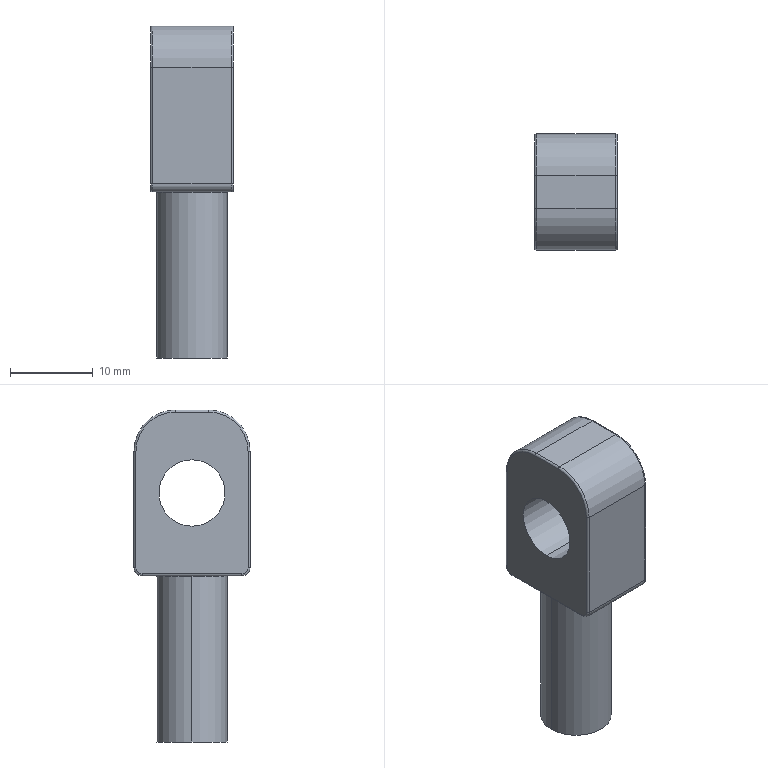Part | SolidWorks | features Cut 1, Extrusion 1, Fillet 1, HoleWzd 1, ICE 1 | 2 solids | 38 faces | box 10 x 14 x 40.005 mm | volume 3250 mm3 | cylinder 18 | plane 8 | torus 8 | cone 4 | commonest cylinder face diameters 0.5 x8 2 x2 2.9 x2 8 x2 8.5 x2 10 x2
STEP:
#1=CARTESIAN_POINT('',(1.45,0.,0.325));
#2=VERTEX_POINT('',#1);
#3=CARTESIAN_POINT('',(-1.45,0.,0.325));
#4=VERTEX_POINT('',#3);
#5=CARTESIAN_POINT('',(0.,0.,0.325));
#6=DIRECTION('',(0.,0.,-1.));
#7=DIRECTION('',(-1.,0.,0.));
#8=AXIS2_PLACEMENT_3D('',#5,#6,#7);
#9=CIRCLE('',#8,1.45);
#10=EDGE_CURVE('',#2,#4,#9,.T.);
#11=ORIENTED_EDGE('',*,*,#10,.F.);
#12=CARTESIAN_POINT('',(1.775,0.,0.));
#13=VERTEX_POINT('',#12);
#14=CARTESIAN_POINT('',(1.775,0.,0.));
#15=DIRECTION('',(0.7071,0.,-0.7071));
#16=VECTOR('',#15,1000.);
#17=LINE('',#14,#16);
#18=EDGE_CURVE('',#2,#13,#17,.T.);
#19=ORIENTED_EDGE('',*,*,#18,.T.);
#20=CARTESIAN_POINT('',(-1.775,0.,0.));
#21=VERTEX_POINT('',#20);
#22=CARTESIAN_POINT('',(0.,0.,0.));
#23=DIRECTION('',(0.,0.,-1.));
#24=DIRECTION('',(-1.,0.,0.));
#25=AXIS2_PLACEMENT_3D('',#22,#23,#24);
#26=CIRCLE('',#25,1.775);
#27=EDGE_CURVE('',#13,#21,#26,.T.);
#28=ORIENTED_EDGE('',*,*,#27,.T.);
#29=CARTESIAN_POINT('',(-1.775,0.,0.));
#30=DIRECTION('',(-0.7071,0.,-0.7071));
#31=VECTOR('',#30,1000.);
#32=LINE('',#29,#31);
#33=EDGE_CURVE('',#4,#21,#32,.T.);
#34=ORIENTED_EDGE('',*,*,#33,.F.);
#35=EDGE_LOOP('',(#11,#19,#28,#34));
#36=FACE_OUTER_BOUND('',#35,.T.);
#37=CARTESIAN_POINT('',(0.,0.,0.));
#38=DIRECTION('',(0.,0.,-1.));
#39=DIRECTION('',(-1.,0.,0.));
#40=AXIS2_PLACEMENT_3D('',#37,#38,#39);
#41=CONICAL_SURFACE('',#40,1.775,0.7854);
#42=ADVANCED_FACE('',(#36),#41,.F.);
#43=CARTESIAN_POINT('',(1.45,0.,10.));
#44=VERTEX_POINT('',#43);
#45=CARTESIAN_POINT('',(-1.45,0.,10.));
#46=VERTEX_POINT('',#45);
#47=CARTESIAN_POINT('',(0.,0.,10.));
#48=DIRECTION('',(0.,0.,-1.));
#49=DIRECTION('',(-1.,0.,0.));
#50=AXIS2_PLACEMENT_3D('',#47,#48,#49);
#51=CIRCLE('',#50,1.45);
#52=EDGE_CURVE('',#44,#46,#51,.T.);
#53=ORIENTED_EDGE('',*,*,#52,.F.);
#54=CARTESIAN_POINT('',(1.45,0.,0.));
#55=DIRECTION('',(0.,0.,-1.));
#56=VECTOR('',#55,1000.);
#57=LINE('',#54,#56);
#58=EDGE_CURVE('',#44,#2,#57,.T.);
#59=ORIENTED_EDGE('',*,*,#58,.T.);
#60=ORIENTED_EDGE('',*,*,#10,.T.);
#61=CARTESIAN_POINT('',(-1.45,0.,0.));
#62=DIRECTION('',(0.,0.,-1.));
#63=VECTOR('',#62,1000.);
#64=LINE('',#61,#63);
#65=EDGE_CURVE('',#46,#4,#64,.T.);
#66=ORIENTED_EDGE('',*,*,#65,.F.);
#67=EDGE_LOOP('',(#53,#59,#60,#66));
#68=FACE_OUTER_BOUND('',#67,.T.);
#69=CARTESIAN_POINT('',(0.,0.,0.));
#70=DIRECTION('',(0.,0.,-1.));
#71=DIRECTION('',(-1.,0.,0.));
#72=AXIS2_PLACEMENT_3D('',#69,#70,#71);
#73=CYLINDRICAL_SURFACE('',#72,1.45);
#74=ADVANCED_FACE('',(#68),#73,.F.);
#75=CARTESIAN_POINT('',(0.,0.,10.871));
#76=VERTEX_POINT('',#75);
#77=CARTESIAN_POINT('',(-1.45,0.,10.));
#78=DIRECTION('',(-0.8572,0.,-0.515));
#79=VECTOR('',#78,1000.);
#80=LINE('',#77,#79);
#81=EDGE_CURVE('',#76,#46,#80,.T.);
#82=ORIENTED_EDGE('',*,*,#81,.F.);
#83=CARTESIAN_POINT('',(1.45,0.,10.));
#84=DIRECTION('',(0.8572,0.,-0.515));
#85=VECTOR('',#84,1000.);
#86=LINE('',#83,#85);
#87=EDGE_CURVE('',#76,#44,#86,.T.);
#88=ORIENTED_EDGE('',*,*,#87,.T.);
#89=ORIENTED_EDGE('',*,*,#52,.T.);
#90=EDGE_LOOP('',(#82,#88,#89));
#91=FACE_OUTER_BOUND('',#90,.T.);
#92=CARTESIAN_POINT('',(0.,0.,10.));
#93=DIRECTION('',(0.,0.,-1.));
#94=DIRECTION('',(-1.,0.,0.));
#95=AXIS2_PLACEMENT_3D('',#92,#93,#94);
#96=CONICAL_SURFACE('',#95,1.45,1.03);
#97=ADVANCED_FACE('',(#91),#96,.F.);
#98=CARTESIAN_POINT('',(4.25,0.,20.));
#99=VERTEX_POINT('',#98);
#100=CARTESIAN_POINT('',(-4.25,0.,20.));
#101=VERTEX_POINT('',#100);
#102=CARTESIAN_POINT('',(0.,0.,20.));
#103=DIRECTION('',(0.,0.,1.));
#104=DIRECTION('',(1.,0.,0.));
#105=AXIS2_PLACEMENT_3D('',#102,#103,#104);
#106=CIRCLE('',#105,4.25);
#107=EDGE_CURVE('',#99,#101,#106,.T.);
#108=ORIENTED_EDGE('',*,*,#107,.F.);
#109=CARTESIAN_POINT('',(4.25,0.,0.));
#110=VERTEX_POINT('',#109);
#111=CARTESIAN_POINT('',(4.25,0.,20.));
#112=DIRECTION('',(0.,0.,-1.));
#113=VECTOR('',#112,1000.);
#114=LINE('',#111,#113);
#115=EDGE_CURVE('',#99,#110,#114,.T.);
#116=ORIENTED_EDGE('',*,*,#115,.T.);
#117=CARTESIAN_POINT('',(-4.25,0.,0.));
#118=VERTEX_POINT('',#117);
#119=CARTESIAN_POINT('',(0.,0.,0.));
#120=DIRECTION('',(0.,0.,1.));
#121=DIRECTION('',(1.,0.,0.));
#122=AXIS2_PLACEMENT_3D('',#119,#120,#121);
#123=CIRCLE('',#122,4.25);
#124=EDGE_CURVE('',#110,#118,#123,.T.);
#125=ORIENTED_EDGE('',*,*,#124,.T.);
#126=CARTESIAN_POINT('',(-4.25,0.,20.));
#127=DIRECTION('',(0.,0.,-1.));
#128=VECTOR('',#127,1000.);
#129=LINE('',#126,#128);
#130=EDGE_CURVE('',#101,#118,#129,.T.);
#131=ORIENTED_EDGE('',*,*,#130,.F.);
#132=EDGE_LOOP('',(#108,#116,#125,#131));
#133=FACE_OUTER_BOUND('',#132,.T.);
#134=CARTESIAN_POINT('',(0.,0.,20.));
#135=DIRECTION('',(0.,0.,-1.));
#136=DIRECTION('',(-1.,0.,0.));
#137=AXIS2_PLACEMENT_3D('',#134,#135,#136);
#138=CYLINDRICAL_SURFACE('',#137,4.25);
#139=ADVANCED_FACE('',(#133),#138,.T.);
#140=ORIENTED_EDGE('',*,*,#115,.F.);
#141=CARTESIAN_POINT('',(0.,0.,20.));
#142=DIRECTION('',(0.,0.,1.));
#143=DIRECTION('',(1.,0.,0.));
#144=AXIS2_PLACEMENT_3D('',#141,#142,#143);
#145=CIRCLE('',#144,4.25);
#146=EDGE_CURVE('',#101,#99,#145,.T.);
#147=ORIENTED_EDGE('',*,*,#146,.F.);
#148=ORIENTED_EDGE('',*,*,#130,.T.);
#149=CARTESIAN_POINT('',(0.,0.,0.));
#150=DIRECTION('',(0.,0.,1.));
#151=DIRECTION('',(1.,0.,0.));
#152=AXIS2_PLACEMENT_3D('',#149,#150,#151);
#153=CIRCLE('',#152,4.25);
#154=EDGE_CURVE('',#118,#110,#153,.T.);
#155=ORIENTED_EDGE('',*,*,#154,.T.);
#156=EDGE_LOOP('',(#140,#147,#148,#155));
#157=FACE_OUTER_BOUND('',#156,.T.);
#158=CARTESIAN_POINT('',(0.,0.,20.));
#159=DIRECTION('',(0.,0.,-1.));
#160=DIRECTION('',(-1.,0.,0.));
#161=AXIS2_PLACEMENT_3D('',#158,#159,#160);
#162=CYLINDRICAL_SURFACE('',#161,4.25);
#163=ADVANCED_FACE('',(#157),#162,.T.);
#164=ORIENTED_EDGE('',*,*,#146,.T.);
#165=ORIENTED_EDGE('',*,*,#107,.T.);
#166=EDGE_LOOP('',(#164,#165));
#167=FACE_OUTER_BOUND('',#166,.T.);
#168=CARTESIAN_POINT('',(0.,0.,20.));
#169=DIRECTION('',(0.,0.,1.));
#170=DIRECTION('',(1.,0.,0.));
#171=AXIS2_PLACEMENT_3D('',#168,#169,#170);
#172=PLANE('',#171);
#173=ADVANCED_FACE('',(#167),#172,.T.);
#174=CARTESIAN_POINT('',(0.,0.,0.));
#175=DIRECTION('',(0.,0.,-1.));
#176=DIRECTION('',(-1.,0.,0.));
#177=AXIS2_PLACEMENT_3D('',#174,#175,#176);
#178=CIRCLE('',#177,1.775);
#179=EDGE_CURVE('',#21,#13,#178,.T.);
#180=ORIENTED_EDGE('',*,*,#179,.F.);
#181=ORIENTED_EDGE('',*,*,#27,.F.);
#182=EDGE_LOOP('',(#180,#181));
#183=FACE_BOUND('',#182,.T.);
#184=ORIENTED_EDGE('',*,*,#154,.F.);
#185=ORIENTED_EDGE('',*,*,#124,.F.);
#186=EDGE_LOOP('',(#184,#185));
#187=FACE_OUTER_BOUND('',#186,.T.);
#188=CARTESIAN_POINT('',(0.,0.,0.));
#189=DIRECTION('',(0.,0.,1.));
#190=DIRECTION('',(1.,0.,0.));
#191=AXIS2_PLACEMENT_3D('',#188,#189,#190);
#192=PLANE('',#191);
#193=ADVANCED_FACE('',(#183,#187),#192,.F.);
#194=ORIENTED_EDGE('',*,*,#87,.F.);
#195=ORIENTED_EDGE('',*,*,#81,.T.);
#196=CARTESIAN_POINT('',(0.,0.,10.));
#197=DIRECTION('',(0.,0.,-1.));
#198=DIRECTION('',(-1.,0.,0.));
#199=AXIS2_PLACEMENT_3D('',#196,#197,#198);
#200=CIRCLE('',#199,1.45);
#201=EDGE_CURVE('',#46,#44,#200,.T.);
#202=ORIENTED_EDGE('',*,*,#201,.T.);
#203=EDGE_LOOP('',(#194,#195,#202));
#204=FACE_OUTER_BOUND('',#203,.T.);
#205=CARTESIAN_POINT('',(0.,0.,10.));
#206=DIRECTION('',(0.,0.,-1.));
#207=DIRECTION('',(-1.,0.,0.));
#208=AXIS2_PLACEMENT_3D('',#205,#206,#207);
#209=CONICAL_SURFACE('',#208,1.45,1.03);
#210=ADVANCED_FACE('',(#204),#209,.F.);
#211=ORIENTED_EDGE('',*,*,#58,.F.);
#212=ORIENTED_EDGE('',*,*,#201,.F.);
#213=ORIENTED_EDGE('',*,*,#65,.T.);
#214=CARTESIAN_POINT('',(0.,0.,0.325));
#215=DIRECTION('',(0.,0.,-1.));
#216=DIRECTION('',(-1.,0.,0.));
#217=AXIS2_PLACEMENT_3D('',#214,#215,#216);
#218=CIRCLE('',#217,1.45);
#219=EDGE_CURVE('',#4,#2,#218,.T.);
#220=ORIENTED_EDGE('',*,*,#219,.T.);
#221=EDGE_LOOP('',(#211,#212,#213,#220));
#222=FACE_OUTER_BOUND('',#221,.T.);
#223=CARTESIAN_POINT('',(0.,0.,0.));
#224=DIRECTION('',(0.,0.,-1.));
#225=DIRECTION('',(-1.,0.,0.));
#226=AXIS2_PLACEMENT_3D('',#223,#224,#225);
#227=CYLINDRICAL_SURFACE('',#226,1.45);
#228=ADVANCED_FACE('',(#222),#227,.F.);
#229=ORIENTED_EDGE('',*,*,#18,.F.);
#230=ORIENTED_EDGE('',*,*,#219,.F.);
#231=ORIENTED_EDGE('',*,*,#33,.T.);
#232=ORIENTED_EDGE('',*,*,#179,.T.);
#233=EDGE_LOOP('',(#229,#230,#231,#232));
#234=FACE_OUTER_BOUND('',#233,.T.);
#235=CARTESIAN_POINT('',(0.,0.,0.));
#236=DIRECTION('',(0.,0.,-1.));
#237=DIRECTION('',(-1.,0.,0.));
#238=AXIS2_PLACEMENT_3D('',#235,#236,#237);
#239=CONICAL_SURFACE('',#238,1.775,0.7854);
#240=ADVANCED_FACE('',(#234),#239,.F.);
#241=CLOSED_SHELL('',(#42,#74,#97,#139,#163,#173,#193,#210,#228,#240));
#242=MANIFOLD_SOLID_BREP('',#241);
#243=CARTESIAN_POINT('',(-5.,0.,34.005));
#244=VERTEX_POINT('',#243);
#245=CARTESIAN_POINT('',(-5.,0.,26.005));
#246=VERTEX_POINT('',#245);
#247=CARTESIAN_POINT('',(-5.,0.,30.005));
#248=DIRECTION('',(1.,0.,0.));
#249=DIRECTION('',(0.,0.,1.));
#250=AXIS2_PLACEMENT_3D('',#247,#248,#249);
#251=CIRCLE('',#250,4.);
#252=EDGE_CURVE('',#244,#246,#251,.T.);
#253=ORIENTED_EDGE('',*,*,#252,.F.);
#254=CARTESIAN_POINT('',(5.,0.,34.005));
#255=VERTEX_POINT('',#254);
#256=CARTESIAN_POINT('',(-5.001,0.,34.005));
#257=DIRECTION('',(1.,0.,0.));
#258=VECTOR('',#257,1000.);
#259=LINE('',#256,#258);
#260=EDGE_CURVE('',#244,#255,#259,.T.);
#261=ORIENTED_EDGE('',*,*,#260,.T.);
#262=CARTESIAN_POINT('',(5.,0.,26.005));
#263=VERTEX_POINT('',#262);
#264=CARTESIAN_POINT('',(5.,0.,30.005));
#265=DIRECTION('',(1.,0.,0.));
#266=DIRECTION('',(0.,0.,-1.));
#267=AXIS2_PLACEMENT_3D('',#264,#265,#266);
#268=CIRCLE('',#267,4.);
#269=EDGE_CURVE('',#255,#263,#268,.T.);
#270=ORIENTED_EDGE('',*,*,#269,.T.);
#271=CARTESIAN_POINT('',(-5.001,0.,26.005));
#272=DIRECTION('',(1.,0.,0.));
#273=VECTOR('',#272,1000.);
#274=LINE('',#271,#273);
#275=EDGE_CURVE('',#246,#263,#274,.T.);
#276=ORIENTED_EDGE('',*,*,#275,.F.);
#277=EDGE_LOOP('',(#253,#261,#270,#276));
#278=FACE_OUTER_BOUND('',#277,.T.);
#279=CARTESIAN_POINT('',(-5.001,0.,30.005));
#280=DIRECTION('',(1.,0.,0.));
#281=DIRECTION('',(0.,0.,-1.));
#282=AXIS2_PLACEMENT_3D('',#279,#280,#281);
#283=CYLINDRICAL_SURFACE('',#282,4.);
#284=ADVANCED_FACE('',(#278),#283,.F.);
#285=CARTESIAN_POINT('',(4.75,-2.,40.005));
#286=VERTEX_POINT('',#285);
#287=CARTESIAN_POINT('',(-4.75,-2.,40.005));
#288=VERTEX_POINT('',#287);
#289=CARTESIAN_POINT('',(5.,-2.,40.005));
#290=DIRECTION('',(-1.,0.,0.));
#291=VECTOR('',#290,1000.);
#292=LINE('',#289,#291);
#293=EDGE_CURVE('',#286,#288,#292,.T.);
#294=ORIENTED_EDGE('',*,*,#293,.T.);
#295=CARTESIAN_POINT('',(-4.75,-7.,35.005));
#296=VERTEX_POINT('',#295);
#297=CARTESIAN_POINT('',(-4.75,-2.,35.005));
#298=DIRECTION('',(1.,0.,0.));
#299=DIRECTION('',(0.,0.,1.));
#300=AXIS2_PLACEMENT_3D('',#297,#298,#299);
#301=CIRCLE('',#300,5.);
#302=EDGE_CURVE('',#288,#296,#301,.T.);
#303=ORIENTED_EDGE('',*,*,#302,.T.);
#304=CARTESIAN_POINT('',(4.75,-7.,35.005));
#305=VERTEX_POINT('',#304);
#306=CARTESIAN_POINT('',(5.,-7.,35.005));
#307=DIRECTION('',(-1.,0.,0.));
#308=VECTOR('',#307,1000.);
#309=LINE('',#306,#308);
#310=EDGE_CURVE('',#305,#296,#309,.T.);
#311=ORIENTED_EDGE('',*,*,#310,.F.);
#312=CARTESIAN_POINT('',(4.75,-2.,35.005));
#313=DIRECTION('',(-1.,0.,0.));
#314=DIRECTION('',(0.,0.,1.));
#315=AXIS2_PLACEMENT_3D('',#312,#313,#314);
#316=CIRCLE('',#315,5.);
#317=EDGE_CURVE('',#305,#286,#316,.T.);
#318=ORIENTED_EDGE('',*,*,#317,.T.);
#319=EDGE_LOOP('',(#294,#303,#311,#318));
#320=FACE_OUTER_BOUND('',#319,.T.);
#321=CARTESIAN_POINT('',(5.,-2.,35.005));
#322=DIRECTION('',(-1.,0.,0.));
#323=DIRECTION('',(0.,0.,1.));
#324=AXIS2_PLACEMENT_3D('',#321,#322,#323);
#325=CYLINDRICAL_SURFACE('',#324,5.);
#326=ADVANCED_FACE('',(#320),#325,.T.);
#327=ORIENTED_EDGE('',*,*,#310,.T.);
#328=CARTESIAN_POINT('',(-4.75,-7.,21.005));
#329=VERTEX_POINT('',#328);
#330=CARTESIAN_POINT('',(-4.75,-7.,21.005));
#331=DIRECTION('',(0.,0.,-1.));
#332=VECTOR('',#331,1000.);
#333=LINE('',#330,#332);
#334=EDGE_CURVE('',#296,#329,#333,.T.);
#335=ORIENTED_EDGE('',*,*,#334,.T.);
#336=CARTESIAN_POINT('',(4.75,-7.,21.005));
#337=VERTEX_POINT('',#336);
#338=CARTESIAN_POINT('',(5.,-7.,21.005));
#339=DIRECTION('',(-1.,0.,0.));
#340=VECTOR('',#339,1000.);
#341=LINE('',#338,#340);
#342=EDGE_CURVE('',#337,#329,#341,.T.);
#343=ORIENTED_EDGE('',*,*,#342,.F.);
#344=CARTESIAN_POINT('',(4.75,-7.,21.005));
#345=DIRECTION('',(0.,0.,1.));
#346=VECTOR('',#345,1000.);
#347=LINE('',#344,#346);
#348=EDGE_CURVE('',#337,#305,#347,.T.);
#349=ORIENTED_EDGE('',*,*,#348,.T.);
#350=EDGE_LOOP('',(#327,#335,#343,#349));
#351=FACE_OUTER_BOUND('',#350,.T.);
#352=CARTESIAN_POINT('',(5.,-7.,21.005));
#353=DIRECTION('',(0.,1.,0.));
#354=DIRECTION('',(0.,0.,1.));
#355=AXIS2_PLACEMENT_3D('',#352,#353,#354);
#356=PLANE('',#355);
#357=ADVANCED_FACE('',(#351),#356,.F.);
#358=ORIENTED_EDGE('',*,*,#342,.T.);
#359=CARTESIAN_POINT('',(-4.75,-6.,20.005));
#360=VERTEX_POINT('',#359);
#361=CARTESIAN_POINT('',(-4.75,-6.,21.005));
#362=DIRECTION('',(1.,0.,0.));
#363=DIRECTION('',(0.,0.,1.));
#364=AXIS2_PLACEMENT_3D('',#361,#362,#363);
#365=CIRCLE('',#364,1.);
#366=EDGE_CURVE('',#329,#360,#365,.T.);
#367=ORIENTED_EDGE('',*,*,#366,.T.);
#368=CARTESIAN_POINT('',(4.75,-6.,20.005));
#369=VERTEX_POINT('',#368);
#370=CARTESIAN_POINT('',(5.,-6.,20.005));
#371=DIRECTION('',(-1.,0.,0.));
#372=VECTOR('',#371,1000.);
#373=LINE('',#370,#372);
#374=EDGE_CURVE('',#369,#360,#373,.T.);
#375=ORIENTED_EDGE('',*,*,#374,.F.);
#376=CARTESIAN_POINT('',(4.75,-6.,21.005));
#377=DIRECTION('',(-1.,0.,0.));
#378=DIRECTION('',(0.,0.,1.));
#379=AXIS2_PLACEMENT_3D('',#376,#377,#378);
#380=CIRCLE('',#379,1.);
#381=EDGE_CURVE('',#369,#337,#380,.T.);
#382=ORIENTED_EDGE('',*,*,#381,.T.);
#383=EDGE_LOOP('',(#358,#367,#375,#382));
#384=FACE_OUTER_BOUND('',#383,.T.);
#385=CARTESIAN_POINT('',(5.,-6.,21.005));
#386=DIRECTION('',(-1.,0.,0.));
#387=DIRECTION('',(0.,0.,1.));
#388=AXIS2_PLACEMENT_3D('',#385,#386,#387);
#389=CYLINDRICAL_SURFACE('',#388,1.);
#390=ADVANCED_FACE('',(#384),#389,.T.);
#391=ORIENTED_EDGE('',*,*,#374,.T.);
#392=CARTESIAN_POINT('',(-4.75,6.,20.005));
#393=VERTEX_POINT('',#392);
#394=CARTESIAN_POINT('',(-4.75,6.,20.005));
#395=DIRECTION('',(0.,1.,0.));
#396=VECTOR('',#395,1000.);
#397=LINE('',#394,#396);
#398=EDGE_CURVE('',#360,#393,#397,.T.);
#399=ORIENTED_EDGE('',*,*,#398,.T.);
#400=CARTESIAN_POINT('',(4.75,6.,20.005));
#401=VERTEX_POINT('',#400);
#402=CARTESIAN_POINT('',(5.,6.,20.005));
#403=DIRECTION('',(-1.,0.,0.));
#404=VECTOR('',#403,1000.);
#405=LINE('',#402,#404);
#406=EDGE_CURVE('',#401,#393,#405,.T.);
#407=ORIENTED_EDGE('',*,*,#406,.F.);
#408=CARTESIAN_POINT('',(4.75,-6.,20.005));
#409=DIRECTION('',(0.,-1.,0.));
#410=VECTOR('',#409,1000.);
#411=LINE('',#408,#410);
#412=EDGE_CURVE('',#401,#369,#411,.T.);
#413=ORIENTED_EDGE('',*,*,#412,.T.);
#414=EDGE_LOOP('',(#391,#399,#407,#413));
#415=FACE_OUTER_BOUND('',#414,.T.);
#416=CARTESIAN_POINT('',(5.,-6.,20.005));
#417=DIRECTION('',(0.,0.,1.));
#418=DIRECTION('',(1.,0.,0.));
#419=AXIS2_PLACEMENT_3D('',#416,#417,#418);
#420=PLANE('',#419);
#421=ADVANCED_FACE('',(#415),#420,.F.);
#422=ORIENTED_EDGE('',*,*,#406,.T.);
#423=CARTESIAN_POINT('',(-4.75,7.,21.005));
#424=VERTEX_POINT('',#423);
#425=CARTESIAN_POINT('',(-4.75,6.,21.005));
#426=DIRECTION('',(1.,0.,0.));
#427=DIRECTION('',(0.,0.,1.));
#428=AXIS2_PLACEMENT_3D('',#425,#426,#427);
#429=CIRCLE('',#428,1.);
#430=EDGE_CURVE('',#393,#424,#429,.T.);
#431=ORIENTED_EDGE('',*,*,#430,.T.);
#432=CARTESIAN_POINT('',(4.75,7.,21.005));
#433=VERTEX_POINT('',#432);
#434=CARTESIAN_POINT('',(5.,7.,21.005));
#435=DIRECTION('',(-1.,0.,0.));
#436=VECTOR('',#435,1000.);
#437=LINE('',#434,#436);
#438=EDGE_CURVE('',#433,#424,#437,.T.);
#439=ORIENTED_EDGE('',*,*,#438,.F.);
#440=CARTESIAN_POINT('',(4.75,6.,21.005));
#441=DIRECTION('',(-1.,0.,0.));
#442=DIRECTION('',(0.,0.,1.));
#443=AXIS2_PLACEMENT_3D('',#440,#441,#442);
#444=CIRCLE('',#443,1.);
#445=EDGE_CURVE('',#433,#401,#444,.T.);
#446=ORIENTED_EDGE('',*,*,#445,.T.);
#447=EDGE_LOOP('',(#422,#431,#439,#446));
#448=FACE_OUTER_BOUND('',#447,.T.);
#449=CARTESIAN_POINT('',(5.,6.,21.005));
#450=DIRECTION('',(-1.,0.,0.));
#451=DIRECTION('',(0.,0.,1.));
#452=AXIS2_PLACEMENT_3D('',#449,#450,#451);
#453=CYLINDRICAL_SURFACE('',#452,1.);
#454=ADVANCED_FACE('',(#448),#453,.T.);
#455=ORIENTED_EDGE('',*,*,#438,.T.);
#456=CARTESIAN_POINT('',(-4.75,7.,35.005));
#457=VERTEX_POINT('',#456);
#458=CARTESIAN_POINT('',(-4.75,7.,35.005));
#459=DIRECTION('',(0.,0.,1.));
#460=VECTOR('',#459,1000.);
#461=LINE('',#458,#460);
#462=EDGE_CURVE('',#424,#457,#461,.T.);
#463=ORIENTED_EDGE('',*,*,#462,.T.);
#464=CARTESIAN_POINT('',(4.75,7.,35.005));
#465=VERTEX_POINT('',#464);
#466=CARTESIAN_POINT('',(5.,7.,35.005));
#467=DIRECTION('',(-1.,0.,0.));
#468=VECTOR('',#467,1000.);
#469=LINE('',#466,#468);
#470=EDGE_CURVE('',#465,#457,#469,.T.);
#471=ORIENTED_EDGE('',*,*,#470,.F.);
#472=CARTESIAN_POINT('',(4.75,7.,21.005));
#473=DIRECTION('',(0.,0.,-1.));
#474=VECTOR('',#473,1000.);
#475=LINE('',#472,#474);
#476=EDGE_CURVE('',#465,#433,#475,.T.);
#477=ORIENTED_EDGE('',*,*,#476,.T.);
#478=EDGE_LOOP('',(#455,#463,#471,#477));
#479=FACE_OUTER_BOUND('',#478,.T.);
#480=CARTESIAN_POINT('',(5.,7.,21.005));
#481=DIRECTION('',(0.,-1.,0.));
#482=DIRECTION('',(0.,0.,-1.));
#483=AXIS2_PLACEMENT_3D('',#480,#481,#482);
#484=PLANE('',#483);
#485=ADVANCED_FACE('',(#479),#484,.F.);
#486=ORIENTED_EDGE('',*,*,#470,.T.);
#487=CARTESIAN_POINT('',(-4.75,2.,40.005));
#488=VERTEX_POINT('',#487);
#489=CARTESIAN_POINT('',(-4.75,2.,35.005));
#490=DIRECTION('',(1.,0.,0.));
#491=DIRECTION('',(0.,0.,1.));
#492=AXIS2_PLACEMENT_3D('',#489,#490,#491);
#493=CIRCLE('',#492,5.);
#494=EDGE_CURVE('',#457,#488,#493,.T.);
#495=ORIENTED_EDGE('',*,*,#494,.T.);
#496=CARTESIAN_POINT('',(4.75,2.,40.005));
#497=VERTEX_POINT('',#496);
#498=CARTESIAN_POINT('',(5.,2.,40.005));
#499=DIRECTION('',(-1.,0.,0.));
#500=VECTOR('',#499,1000.);
#501=LINE('',#498,#500);
#502=EDGE_CURVE('',#497,#488,#501,.T.);
#503=ORIENTED_EDGE('',*,*,#502,.F.);
#504=CARTESIAN_POINT('',(4.75,2.,35.005));
#505=DIRECTION('',(-1.,0.,0.));
#506=DIRECTION('',(0.,0.,1.));
#507=AXIS2_PLACEMENT_3D('',#504,#505,#506);
#508=CIRCLE('',#507,5.);
#509=EDGE_CURVE('',#497,#465,#508,.T.);
#510=ORIENTED_EDGE('',*,*,#509,.T.);
#511=EDGE_LOOP('',(#486,#495,#503,#510));
#512=FACE_OUTER_BOUND('',#511,.T.);
#513=CARTESIAN_POINT('',(5.,2.,35.005));
#514=DIRECTION('',(-1.,0.,0.));
#515=DIRECTION('',(0.,0.,1.));
#516=AXIS2_PLACEMENT_3D('',#513,#514,#515);
#517=CYLINDRICAL_SURFACE('',#516,5.);
#518=ADVANCED_FACE('',(#512),#517,.T.);
#519=ORIENTED_EDGE('',*,*,#502,.T.);
#520=CARTESIAN_POINT('',(-4.75,-2.,40.005));
#521=DIRECTION('',(0.,-1.,0.));
#522=VECTOR('',#521,1000.);
#523=LINE('',#520,#522);
#524=EDGE_CURVE('',#488,#288,#523,.T.);
#525=ORIENTED_EDGE('',*,*,#524,.T.);
#526=ORIENTED_EDGE('',*,*,#293,.F.);
#527=CARTESIAN_POINT('',(4.75,-2.,40.005));
#528=DIRECTION('',(0.,1.,0.));
#529=VECTOR('',#528,1000.);
#530=LINE('',#527,#529);
#531=EDGE_CURVE('',#286,#497,#530,.T.);
#532=ORIENTED_EDGE('',*,*,#531,.T.);
#533=EDGE_LOOP('',(#519,#525,#526,#532));
#534=FACE_OUTER_BOUND('',#533,.T.);
#535=CARTESIAN_POINT('',(5.,-2.,40.005));
#536=DIRECTION('',(0.,0.,-1.));
#537=DIRECTION('',(-1.,0.,0.));
#538=AXIS2_PLACEMENT_3D('',#535,#536,#537);
#539=PLANE('',#538);
#540=ADVANCED_FACE('',(#534),#539,.F.);
#541=CARTESIAN_POINT('',(5.,0.,30.005));
#542=DIRECTION('',(1.,0.,0.));
#543=DIRECTION('',(0.,0.,-1.));
#544=AXIS2_PLACEMENT_3D('',#541,#542,#543);
#545=CIRCLE('',#544,4.);
#546=EDGE_CURVE('',#263,#255,#545,.T.);
#547=ORIENTED_EDGE('',*,*,#546,.F.);
#548=ORIENTED_EDGE('',*,*,#269,.F.);
#549=EDGE_LOOP('',(#547,#548));
#550=FACE_BOUND('',#549,.T.);
#551=CARTESIAN_POINT('',(5.,6.75,35.005));
#552=VERTEX_POINT('',#551);
#553=CARTESIAN_POINT('',(5.,2.,39.755));
#554=VERTEX_POINT('',#553);
#555=CARTESIAN_POINT('',(5.,2.,35.005));
#556=DIRECTION('',(1.,0.,0.));
#557=DIRECTION('',(0.,0.,1.));
#558=AXIS2_PLACEMENT_3D('',#555,#556,#557);
#559=CIRCLE('',#558,4.75);
#560=EDGE_CURVE('',#552,#554,#559,.T.);
#561=ORIENTED_EDGE('',*,*,#560,.T.);
#562=CARTESIAN_POINT('',(5.,-2.,39.755));
#563=VERTEX_POINT('',#562);
#564=CARTESIAN_POINT('',(5.,-2.,39.755));
#565=DIRECTION('',(0.,-1.,0.));
#566=VECTOR('',#565,1000.);
#567=LINE('',#564,#566);
#568=EDGE_CURVE('',#554,#563,#567,.T.);
#569=ORIENTED_EDGE('',*,*,#568,.T.);
#570=CARTESIAN_POINT('',(5.,-6.75,35.005));
#571=VERTEX_POINT('',#570);
#572=CARTESIAN_POINT('',(5.,-2.,35.005));
#573=DIRECTION('',(1.,0.,0.));
#574=DIRECTION('',(0.,0.,1.));
#575=AXIS2_PLACEMENT_3D('',#572,#573,#574);
#576=CIRCLE('',#575,4.75);
#577=EDGE_CURVE('',#563,#571,#576,.T.);
#578=ORIENTED_EDGE('',*,*,#577,.T.);
#579=CARTESIAN_POINT('',(5.,-6.75,21.005));
#580=VERTEX_POINT('',#579);
#581=CARTESIAN_POINT('',(5.,-6.75,35.005));
#582=DIRECTION('',(0.,0.,-1.));
#583=VECTOR('',#582,1000.);
#584=LINE('',#581,#583);
#585=EDGE_CURVE('',#571,#580,#584,.T.);
#586=ORIENTED_EDGE('',*,*,#585,.T.);
#587=CARTESIAN_POINT('',(5.,-6.,20.255));
#588=VERTEX_POINT('',#587);
#589=CARTESIAN_POINT('',(5.,-6.,21.005));
#590=DIRECTION('',(1.,0.,0.));
#591=DIRECTION('',(0.,0.,1.));
#592=AXIS2_PLACEMENT_3D('',#589,#590,#591);
#593=CIRCLE('',#592,0.75);
#594=EDGE_CURVE('',#580,#588,#593,.T.);
#595=ORIENTED_EDGE('',*,*,#594,.T.);
#596=CARTESIAN_POINT('',(5.,6.,20.255));
#597=VERTEX_POINT('',#596);
#598=CARTESIAN_POINT('',(5.,-2.,20.255));
#599=DIRECTION('',(0.,1.,0.));
#600=VECTOR('',#599,1000.);
#601=LINE('',#598,#600);
#602=EDGE_CURVE('',#588,#597,#601,.T.);
#603=ORIENTED_EDGE('',*,*,#602,.T.);
#604=CARTESIAN_POINT('',(5.,6.75,21.005));
#605=VERTEX_POINT('',#604);
#606=CARTESIAN_POINT('',(5.,6.,21.005));
#607=DIRECTION('',(1.,0.,0.));
#608=DIRECTION('',(0.,0.,1.));
#609=AXIS2_PLACEMENT_3D('',#606,#607,#608);
#610=CIRCLE('',#609,0.75);
#611=EDGE_CURVE('',#597,#605,#610,.T.);
#612=ORIENTED_EDGE('',*,*,#611,.T.);
#613=CARTESIAN_POINT('',(5.,6.75,35.005));
#614=DIRECTION('',(0.,0.,1.));
#615=VECTOR('',#614,1000.);
#616=LINE('',#613,#615);
#617=EDGE_CURVE('',#605,#552,#616,.T.);
#618=ORIENTED_EDGE('',*,*,#617,.T.);
#619=EDGE_LOOP('',(#561,#569,#578,#586,#595,#603,#612,#618));
#620=FACE_OUTER_BOUND('',#619,.T.);
#621=CARTESIAN_POINT('',(5.,-2.,35.005));
#622=DIRECTION('',(-1.,0.,0.));
#623=DIRECTION('',(0.,0.,1.));
#624=AXIS2_PLACEMENT_3D('',#621,#622,#623);
#625=PLANE('',#624);
#626=ADVANCED_FACE('',(#550,#620),#625,.F.);
#627=CARTESIAN_POINT('',(-5.,0.,30.005));
#628=DIRECTION('',(1.,0.,0.));
#629=DIRECTION('',(0.,0.,1.));
#630=AXIS2_PLACEMENT_3D('',#627,#628,#629);
#631=CIRCLE('',#630,4.);
#632=EDGE_CURVE('',#246,#244,#631,.T.);
#633=ORIENTED_EDGE('',*,*,#632,.T.);
#634=ORIENTED_EDGE('',*,*,#252,.T.);
#635=EDGE_LOOP('',(#633,#634));
#636=FACE_BOUND('',#635,.T.);
#637=CARTESIAN_POINT('',(-5.,-6.,20.255));
#638=VERTEX_POINT('',#637);
#639=CARTESIAN_POINT('',(-5.,-6.75,21.005));
#640=VERTEX_POINT('',#639);
#641=CARTESIAN_POINT('',(-5.,-6.,21.005));
#642=DIRECTION('',(-1.,0.,0.));
#643=DIRECTION('',(0.,0.,1.));
#644=AXIS2_PLACEMENT_3D('',#641,#642,#643);
#645=CIRCLE('',#644,0.75);
#646=EDGE_CURVE('',#638,#640,#645,.T.);
#647=ORIENTED_EDGE('',*,*,#646,.T.);
#648=CARTESIAN_POINT('',(-5.,-6.75,35.005));
#649=VERTEX_POINT('',#648);
#650=CARTESIAN_POINT('',(-5.,-6.75,35.005));
#651=DIRECTION('',(0.,0.,1.));
#652=VECTOR('',#651,1000.);
#653=LINE('',#650,#652);
#654=EDGE_CURVE('',#640,#649,#653,.T.);
#655=ORIENTED_EDGE('',*,*,#654,.T.);
#656=CARTESIAN_POINT('',(-5.,-2.,39.755));
#657=VERTEX_POINT('',#656);
#658=CARTESIAN_POINT('',(-5.,-2.,35.005));
#659=DIRECTION('',(-1.,0.,0.));
#660=DIRECTION('',(0.,0.,1.));
#661=AXIS2_PLACEMENT_3D('',#658,#659,#660);
#662=CIRCLE('',#661,4.75);
#663=EDGE_CURVE('',#649,#657,#662,.T.);
#664=ORIENTED_EDGE('',*,*,#663,.T.);
#665=CARTESIAN_POINT('',(-5.,2.,39.755));
#666=VERTEX_POINT('',#665);
#667=CARTESIAN_POINT('',(-5.,2.,39.755));
#668=DIRECTION('',(0.,1.,0.));
#669=VECTOR('',#668,1000.);
#670=LINE('',#667,#669);
#671=EDGE_CURVE('',#657,#666,#670,.T.);
#672=ORIENTED_EDGE('',*,*,#671,.T.);
#673=CARTESIAN_POINT('',(-5.,6.75,35.005));
#674=VERTEX_POINT('',#673);
#675=CARTESIAN_POINT('',(-5.,2.,35.005));
#676=DIRECTION('',(-1.,0.,0.));
#677=DIRECTION('',(0.,0.,1.));
#678=AXIS2_PLACEMENT_3D('',#675,#676,#677);
#679=CIRCLE('',#678,4.75);
#680=EDGE_CURVE('',#666,#674,#679,.T.);
#681=ORIENTED_EDGE('',*,*,#680,.T.);
#682=CARTESIAN_POINT('',(-5.,6.75,21.005));
#683=VERTEX_POINT('',#682);
#684=CARTESIAN_POINT('',(-5.,6.75,21.005));
#685=DIRECTION('',(0.,0.,-1.));
#686=VECTOR('',#685,1000.);
#687=LINE('',#684,#686);
#688=EDGE_CURVE('',#674,#683,#687,.T.);
#689=ORIENTED_EDGE('',*,*,#688,.T.);
#690=CARTESIAN_POINT('',(-5.,6.,20.255));
#691=VERTEX_POINT('',#690);
#692=CARTESIAN_POINT('',(-5.,6.,21.005));
#693=DIRECTION('',(-1.,0.,0.));
#694=DIRECTION('',(0.,0.,1.));
#695=AXIS2_PLACEMENT_3D('',#692,#693,#694);
#696=CIRCLE('',#695,0.75);
#697=EDGE_CURVE('',#683,#691,#696,.T.);
#698=ORIENTED_EDGE('',*,*,#697,.T.);
#699=CARTESIAN_POINT('',(-5.,-6.,20.255));
#700=DIRECTION('',(0.,-1.,0.));
#701=VECTOR('',#700,1000.);
#702=LINE('',#699,#701);
#703=EDGE_CURVE('',#691,#638,#702,.T.);
#704=ORIENTED_EDGE('',*,*,#703,.T.);
#705=EDGE_LOOP('',(#647,#655,#664,#672,#681,#689,#698,#704));
#706=FACE_OUTER_BOUND('',#705,.T.);
#707=CARTESIAN_POINT('',(-5.,-2.,35.005));
#708=DIRECTION('',(-1.,0.,0.));
#709=DIRECTION('',(0.,0.,1.));
#710=AXIS2_PLACEMENT_3D('',#707,#708,#709);
#711=PLANE('',#710);
#712=ADVANCED_FACE('',(#636,#706),#711,.T.);
#713=CARTESIAN_POINT('',(-4.75,6.75,21.005));
#714=DIRECTION('',(0.,0.,-1.));
#715=DIRECTION('',(0.,1.,0.));
#716=AXIS2_PLACEMENT_3D('',#713,#714,#715);
#717=CIRCLE('',#716,0.25);
#718=EDGE_CURVE('',#683,#424,#717,.T.);
#719=ORIENTED_EDGE('',*,*,#718,.F.);
#720=ORIENTED_EDGE('',*,*,#688,.F.);
#721=CARTESIAN_POINT('',(-4.75,6.75,35.005));
#722=DIRECTION('',(0.,0.,1.));
#723=DIRECTION('',(1.,0.,0.));
#724=AXIS2_PLACEMENT_3D('',#721,#722,#723);
#725=CIRCLE('',#724,0.25);
#726=EDGE_CURVE('',#457,#674,#725,.T.);
#727=ORIENTED_EDGE('',*,*,#726,.F.);
#728=ORIENTED_EDGE('',*,*,#462,.F.);
#729=EDGE_LOOP('',(#719,#720,#727,#728));
#730=FACE_OUTER_BOUND('',#729,.T.);
#731=CARTESIAN_POINT('',(-4.75,6.75,21.005));
#732=DIRECTION('',(0.,0.,-1.));
#733=DIRECTION('',(0.,1.,0.));
#734=AXIS2_PLACEMENT_3D('',#731,#732,#733);
#735=CYLINDRICAL_SURFACE('',#734,0.25);
#736=ADVANCED_FACE('',(#730),#735,.T.);
#737=ORIENTED_EDGE('',*,*,#726,.T.);
#738=ORIENTED_EDGE('',*,*,#680,.F.);
#739=CARTESIAN_POINT('',(-4.75,2.,39.755));
#740=DIRECTION('',(0.,-1.,0.));
#741=DIRECTION('',(0.,0.,-1.));
#742=AXIS2_PLACEMENT_3D('',#739,#740,#741);
#743=CIRCLE('',#742,0.25);
#744=EDGE_CURVE('',#488,#666,#743,.T.);
#745=ORIENTED_EDGE('',*,*,#744,.F.);
#746=ORIENTED_EDGE('',*,*,#494,.F.);
#747=EDGE_LOOP('',(#737,#738,#745,#746));
#748=FACE_OUTER_BOUND('',#747,.T.);
#749=CARTESIAN_POINT('',(-4.75,2.,35.005));
#750=DIRECTION('',(-1.,0.,0.));
#751=DIRECTION('',(0.,0.,1.));
#752=AXIS2_PLACEMENT_3D('',#749,#750,#751);
#753=TOROIDAL_SURFACE('',#752,4.75,0.25);
#754=ADVANCED_FACE('',(#748),#753,.T.);
#755=ORIENTED_EDGE('',*,*,#718,.T.);
#756=ORIENTED_EDGE('',*,*,#430,.F.);
#757=CARTESIAN_POINT('',(-4.75,6.,20.255));
#758=DIRECTION('',(0.,-1.,0.));
#759=DIRECTION('',(0.,0.,-1.));
#760=AXIS2_PLACEMENT_3D('',#757,#758,#759);
#761=CIRCLE('',#760,0.25);
#762=EDGE_CURVE('',#691,#393,#761,.T.);
#763=ORIENTED_EDGE('',*,*,#762,.F.);
#764=ORIENTED_EDGE('',*,*,#697,.F.);
#765=EDGE_LOOP('',(#755,#756,#763,#764));
#766=FACE_OUTER_BOUND('',#765,.T.);
#767=CARTESIAN_POINT('',(-4.75,6.,21.005));
#768=DIRECTION('',(-1.,0.,0.));
#769=DIRECTION('',(0.,0.,1.));
#770=AXIS2_PLACEMENT_3D('',#767,#768,#769);
#771=TOROIDAL_SURFACE('',#770,0.75,0.25);
#772=ADVANCED_FACE('',(#766),#771,.T.);
#773=ORIENTED_EDGE('',*,*,#744,.T.);
#774=ORIENTED_EDGE('',*,*,#671,.F.);
#775=CARTESIAN_POINT('',(-4.75,-2.,39.755));
#776=DIRECTION('',(0.,-1.,0.));
#777=DIRECTION('',(0.,0.,-1.));
#778=AXIS2_PLACEMENT_3D('',#775,#776,#777);
#779=CIRCLE('',#778,0.25);
#780=EDGE_CURVE('',#288,#657,#779,.T.);
#781=ORIENTED_EDGE('',*,*,#780,.F.);
#782=ORIENTED_EDGE('',*,*,#524,.F.);
#783=EDGE_LOOP('',(#773,#774,#781,#782));
#784=FACE_OUTER_BOUND('',#783,.T.);
#785=CARTESIAN_POINT('',(-4.75,-2.,39.755));
#786=DIRECTION('',(0.,1.,0.));
#787=DIRECTION('',(0.,0.,1.));
#788=AXIS2_PLACEMENT_3D('',#785,#786,#787);
#789=CYLINDRICAL_SURFACE('',#788,0.25);
#790=ADVANCED_FACE('',(#784),#789,.T.);
#791=ORIENTED_EDGE('',*,*,#762,.T.);
#792=ORIENTED_EDGE('',*,*,#398,.F.);
#793=CARTESIAN_POINT('',(-4.75,-6.,20.255));
#794=DIRECTION('',(0.,-1.,0.));
#795=DIRECTION('',(0.,0.,-1.));
#796=AXIS2_PLACEMENT_3D('',#793,#794,#795);
#797=CIRCLE('',#796,0.25);
#798=EDGE_CURVE('',#638,#360,#797,.T.);
#799=ORIENTED_EDGE('',*,*,#798,.F.);
#800=ORIENTED_EDGE('',*,*,#703,.F.);
#801=EDGE_LOOP('',(#791,#792,#799,#800));
#802=FACE_OUTER_BOUND('',#801,.T.);
#803=CARTESIAN_POINT('',(-4.75,-6.,20.255));
#804=DIRECTION('',(0.,-1.,0.));
#805=DIRECTION('',(0.,0.,-1.));
#806=AXIS2_PLACEMENT_3D('',#803,#804,#805);
#807=CYLINDRICAL_SURFACE('',#806,0.25);
#808=ADVANCED_FACE('',(#802),#807,.T.);
#809=ORIENTED_EDGE('',*,*,#780,.T.);
#810=ORIENTED_EDGE('',*,*,#663,.F.);
#811=CARTESIAN_POINT('',(-4.75,-6.75,35.005));
#812=DIRECTION('',(0.,0.,-1.));
#813=DIRECTION('',(-1.,0.,0.));
#814=AXIS2_PLACEMENT_3D('',#811,#812,#813);
#815=CIRCLE('',#814,0.25);
#816=EDGE_CURVE('',#296,#649,#815,.T.);
#817=ORIENTED_EDGE('',*,*,#816,.F.);
#818=ORIENTED_EDGE('',*,*,#302,.F.);
#819=EDGE_LOOP('',(#809,#810,#817,#818));
#820=FACE_OUTER_BOUND('',#819,.T.);
#821=CARTESIAN_POINT('',(-4.75,-2.,35.005));
#822=DIRECTION('',(-1.,0.,0.));
#823=DIRECTION('',(0.,0.,1.));
#824=AXIS2_PLACEMENT_3D('',#821,#822,#823);
#825=TOROIDAL_SURFACE('',#824,4.75,0.25);
#826=ADVANCED_FACE('',(#820),#825,.T.);
#827=ORIENTED_EDGE('',*,*,#798,.T.);
#828=ORIENTED_EDGE('',*,*,#366,.F.);
#829=CARTESIAN_POINT('',(-4.75,-6.75,21.005));
#830=DIRECTION('',(0.,0.,1.));
#831=DIRECTION('',(1.,0.,0.));
#832=AXIS2_PLACEMENT_3D('',#829,#830,#831);
#833=CIRCLE('',#832,0.25);
#834=EDGE_CURVE('',#640,#329,#833,.T.);
#835=ORIENTED_EDGE('',*,*,#834,.F.);
#836=ORIENTED_EDGE('',*,*,#646,.F.);
#837=EDGE_LOOP('',(#827,#828,#835,#836));
#838=FACE_OUTER_BOUND('',#837,.T.);
#839=CARTESIAN_POINT('',(-4.75,-6.,21.005));
#840=DIRECTION('',(-1.,0.,0.));
#841=DIRECTION('',(0.,0.,1.));
#842=AXIS2_PLACEMENT_3D('',#839,#840,#841);
#843=TOROIDAL_SURFACE('',#842,0.75,0.25);
#844=ADVANCED_FACE('',(#838),#843,.T.);
#845=ORIENTED_EDGE('',*,*,#816,.T.);
#846=ORIENTED_EDGE('',*,*,#654,.F.);
#847=ORIENTED_EDGE('',*,*,#834,.T.);
#848=ORIENTED_EDGE('',*,*,#334,.F.);
#849=EDGE_LOOP('',(#845,#846,#847,#848));
#850=FACE_OUTER_BOUND('',#849,.T.);
#851=CARTESIAN_POINT('',(-4.75,-6.75,21.005));
#852=DIRECTION('',(0.,0.,1.));
#853=DIRECTION('',(0.,-1.,0.));
#854=AXIS2_PLACEMENT_3D('',#851,#852,#853);
#855=CYLINDRICAL_SURFACE('',#854,0.25);
#856=ADVANCED_FACE('',(#850),#855,.T.);
#857=CARTESIAN_POINT('',(4.75,-6.,20.255));
#858=DIRECTION('',(0.,-1.,0.));
#859=DIRECTION('',(0.,0.,-1.));
#860=AXIS2_PLACEMENT_3D('',#857,#858,#859);
#861=CIRCLE('',#860,0.25);
#862=EDGE_CURVE('',#369,#588,#861,.T.);
#863=ORIENTED_EDGE('',*,*,#862,.F.);
#864=ORIENTED_EDGE('',*,*,#412,.F.);
#865=CARTESIAN_POINT('',(4.75,6.,20.255));
#866=DIRECTION('',(0.,1.,0.));
#867=DIRECTION('',(0.,0.,1.));
#868=AXIS2_PLACEMENT_3D('',#865,#866,#867);
#869=CIRCLE('',#868,0.25);
#870=EDGE_CURVE('',#597,#401,#869,.T.);
#871=ORIENTED_EDGE('',*,*,#870,.F.);
#872=ORIENTED_EDGE('',*,*,#602,.F.);
#873=EDGE_LOOP('',(#863,#864,#871,#872));
#874=FACE_OUTER_BOUND('',#873,.T.);
#875=CARTESIAN_POINT('',(4.75,-2.,20.255));
#876=DIRECTION('',(0.,1.,0.));
#877=DIRECTION('',(0.,0.,1.));
#878=AXIS2_PLACEMENT_3D('',#875,#876,#877);
#879=CYLINDRICAL_SURFACE('',#878,0.25);
#880=ADVANCED_FACE('',(#874),#879,.T.);
#881=ORIENTED_EDGE('',*,*,#870,.T.);
#882=ORIENTED_EDGE('',*,*,#445,.F.);
#883=CARTESIAN_POINT('',(4.75,6.75,21.005));
#884=DIRECTION('',(0.,0.,1.));
#885=DIRECTION('',(1.,0.,0.));
#886=AXIS2_PLACEMENT_3D('',#883,#884,#885);
#887=CIRCLE('',#886,0.25);
#888=EDGE_CURVE('',#605,#433,#887,.T.);
#889=ORIENTED_EDGE('',*,*,#888,.F.);
#890=ORIENTED_EDGE('',*,*,#611,.F.);
#891=EDGE_LOOP('',(#881,#882,#889,#890));
#892=FACE_OUTER_BOUND('',#891,.T.);
#893=CARTESIAN_POINT('',(4.75,6.,21.005));
#894=DIRECTION('',(-1.,0.,0.));
#895=DIRECTION('',(0.,0.,1.));
#896=AXIS2_PLACEMENT_3D('',#893,#894,#895);
#897=TOROIDAL_SURFACE('',#896,0.75,0.25);
#898=ADVANCED_FACE('',(#892),#897,.T.);
#899=ORIENTED_EDGE('',*,*,#862,.T.);
#900=ORIENTED_EDGE('',*,*,#594,.F.);
#901=CARTESIAN_POINT('',(4.75,-6.75,21.005));
#902=DIRECTION('',(0.,0.,1.));
#903=DIRECTION('',(0.,-1.,0.));
#904=AXIS2_PLACEMENT_3D('',#901,#902,#903);
#905=CIRCLE('',#904,0.25);
#906=EDGE_CURVE('',#337,#580,#905,.T.);
#907=ORIENTED_EDGE('',*,*,#906,.F.);
#908=ORIENTED_EDGE('',*,*,#381,.F.);
#909=EDGE_LOOP('',(#899,#900,#907,#908));
#910=FACE_OUTER_BOUND('',#909,.T.);
#911=CARTESIAN_POINT('',(4.75,-6.,21.005));
#912=DIRECTION('',(-1.,0.,0.));
#913=DIRECTION('',(0.,0.,1.));
#914=AXIS2_PLACEMENT_3D('',#911,#912,#913);
#915=TOROIDAL_SURFACE('',#914,0.75,0.25);
#916=ADVANCED_FACE('',(#910),#915,.T.);
#917=ORIENTED_EDGE('',*,*,#888,.T.);
#918=ORIENTED_EDGE('',*,*,#476,.F.);
#919=CARTESIAN_POINT('',(4.75,6.75,35.005));
#920=DIRECTION('',(0.,0.,1.));
#921=DIRECTION('',(1.,0.,0.));
#922=AXIS2_PLACEMENT_3D('',#919,#920,#921);
#923=CIRCLE('',#922,0.25);
#924=EDGE_CURVE('',#552,#465,#923,.T.);
#925=ORIENTED_EDGE('',*,*,#924,.F.);
#926=ORIENTED_EDGE('',*,*,#617,.F.);
#927=EDGE_LOOP('',(#917,#918,#925,#926));
#928=FACE_OUTER_BOUND('',#927,.T.);
#929=CARTESIAN_POINT('',(4.75,6.75,35.005));
#930=DIRECTION('',(0.,0.,1.));
#931=DIRECTION('',(0.,-1.,0.));
#932=AXIS2_PLACEMENT_3D('',#929,#930,#931);
#933=CYLINDRICAL_SURFACE('',#932,0.25);
#934=ADVANCED_FACE('',(#928),#933,.T.);
#935=ORIENTED_EDGE('',*,*,#906,.T.);
#936=ORIENTED_EDGE('',*,*,#585,.F.);
#937=CARTESIAN_POINT('',(4.75,-6.75,35.005));
#938=DIRECTION('',(0.,0.,1.));
#939=DIRECTION('',(1.,0.,0.));
#940=AXIS2_PLACEMENT_3D('',#937,#938,#939);
#941=CIRCLE('',#940,0.25);
#942=EDGE_CURVE('',#305,#571,#941,.T.);
#943=ORIENTED_EDGE('',*,*,#942,.F.);
#944=ORIENTED_EDGE('',*,*,#348,.F.);
#945=EDGE_LOOP('',(#935,#936,#943,#944));
#946=FACE_OUTER_BOUND('',#945,.T.);
#947=CARTESIAN_POINT('',(4.75,-6.75,35.005));
#948=DIRECTION('',(0.,0.,-1.));
#949=DIRECTION('',(0.,1.,0.));
#950=AXIS2_PLACEMENT_3D('',#947,#948,#949);
#951=CYLINDRICAL_SURFACE('',#950,0.25);
#952=ADVANCED_FACE('',(#946),#951,.T.);
#953=ORIENTED_EDGE('',*,*,#924,.T.);
#954=ORIENTED_EDGE('',*,*,#509,.F.);
#955=CARTESIAN_POINT('',(4.75,2.,39.755));
#956=DIRECTION('',(0.,-1.,0.));
#957=DIRECTION('',(0.,0.,-1.));
#958=AXIS2_PLACEMENT_3D('',#955,#956,#957);
#959=CIRCLE('',#958,0.25);
#960=EDGE_CURVE('',#554,#497,#959,.T.);
#961=ORIENTED_EDGE('',*,*,#960,.F.);
#962=ORIENTED_EDGE('',*,*,#560,.F.);
#963=EDGE_LOOP('',(#953,#954,#961,#962));
#964=FACE_OUTER_BOUND('',#963,.T.);
#965=CARTESIAN_POINT('',(4.75,2.,35.005));
#966=DIRECTION('',(-1.,0.,0.));
#967=DIRECTION('',(0.,0.,1.));
#968=AXIS2_PLACEMENT_3D('',#965,#966,#967);
#969=TOROIDAL_SURFACE('',#968,4.75,0.25);
#970=ADVANCED_FACE('',(#964),#969,.T.);
#971=ORIENTED_EDGE('',*,*,#942,.T.);
#972=ORIENTED_EDGE('',*,*,#577,.F.);
#973=CARTESIAN_POINT('',(4.75,-2.,39.755));
#974=DIRECTION('',(0.,1.,0.));
#975=DIRECTION('',(0.,0.,1.));
#976=AXIS2_PLACEMENT_3D('',#973,#974,#975);
#977=CIRCLE('',#976,0.25);
#978=EDGE_CURVE('',#286,#563,#977,.T.);
#979=ORIENTED_EDGE('',*,*,#978,.F.);
#980=ORIENTED_EDGE('',*,*,#317,.F.);
#981=EDGE_LOOP('',(#971,#972,#979,#980));
#982=FACE_OUTER_BOUND('',#981,.T.);
#983=CARTESIAN_POINT('',(4.75,-2.,35.005));
#984=DIRECTION('',(-1.,0.,0.));
#985=DIRECTION('',(0.,0.,1.));
#986=AXIS2_PLACEMENT_3D('',#983,#984,#985);
#987=TOROIDAL_SURFACE('',#986,4.75,0.25);
#988=ADVANCED_FACE('',(#982),#987,.T.);
#989=ORIENTED_EDGE('',*,*,#960,.T.);
#990=ORIENTED_EDGE('',*,*,#531,.F.);
#991=ORIENTED_EDGE('',*,*,#978,.T.);
#992=ORIENTED_EDGE('',*,*,#568,.F.);
#993=EDGE_LOOP('',(#989,#990,#991,#992));
#994=FACE_OUTER_BOUND('',#993,.T.);
#995=CARTESIAN_POINT('',(4.75,-2.,39.755));
#996=DIRECTION('',(0.,-1.,0.));
#997=DIRECTION('',(0.,0.,-1.));
#998=AXIS2_PLACEMENT_3D('',#995,#996,#997);
#999=CYLINDRICAL_SURFACE('',#998,0.25);
#1000=ADVANCED_FACE('',(#994),#999,.T.);
#1001=ORIENTED_EDGE('',*,*,#260,.F.);
#1002=ORIENTED_EDGE('',*,*,#632,.F.);
#1003=ORIENTED_EDGE('',*,*,#275,.T.);
#1004=ORIENTED_EDGE('',*,*,#546,.T.);
#1005=EDGE_LOOP('',(#1001,#1002,#1003,#1004));
#1006=FACE_OUTER_BOUND('',#1005,.T.);
#1007=CARTESIAN_POINT('',(-5.001,0.,30.005));
#1008=DIRECTION('',(1.,0.,0.));
#1009=DIRECTION('',(0.,0.,-1.));
#1010=AXIS2_PLACEMENT_3D('',#1007,#1008,#1009);
#1011=CYLINDRICAL_SURFACE('',#1010,4.);
#1012=ADVANCED_FACE('',(#1006),#1011,.F.);
#1013=CLOSED_SHELL('',(#284,#326,#357,#390,#421,#454,#485,#518,#540,#626,#712,#736,#754,#772,#790,#808,#826,#844,#856,#880,#898,#916,#934,#952,#970,#988,#1000,#1012));
#1014=MANIFOLD_SOLID_BREP('',#1013);
#1015=CARTESIAN_POINT('',(0.,0.,0.));
#1016=DIRECTION('',(0.,0.,1.));
#1017=DIRECTION('',(1.,0.,0.));
#1018=AXIS2_PLACEMENT_3D('',#1015,#1016,#1017);
#1019=(LENGTH_UNIT()NAMED_UNIT(*)SI_UNIT(.MILLI.,.METRE.));
#1020=UNCERTAINTY_MEASURE_WITH_UNIT(LENGTH_MEASURE(0.00001),#1019,'','');
#1021=(NAMED_UNIT(*)PLANE_ANGLE_UNIT()SI_UNIT($,.RADIAN.));
#1022=(NAMED_UNIT(*)SI_UNIT($,.STERADIAN.)SOLID_ANGLE_UNIT());
#1023=(GEOMETRIC_REPRESENTATION_CONTEXT(3)GLOBAL_UNCERTAINTY_ASSIGNED_CONTEXT((#1020))GLOBAL_UNIT_ASSIGNED_CONTEXT((#1019,#1021,#1022))REPRESENTATION_CONTEXT('',''));
#1024=ADVANCED_BREP_SHAPE_REPRESENTATION('',(#242,#1014,#1018),#1023);